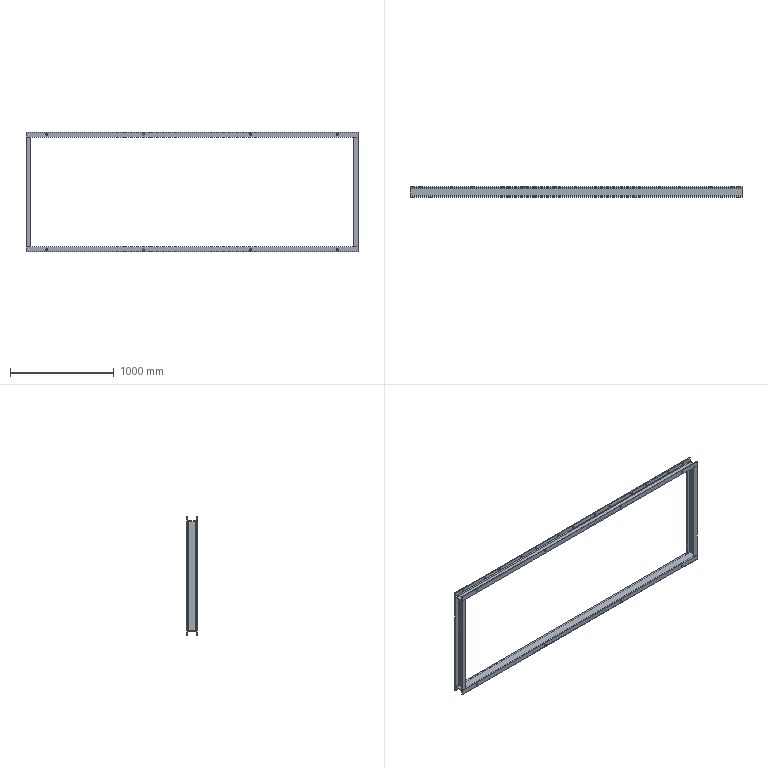Part | STEP file | SW-102-Base1_default<by machining> | 4 solids | 124 faces | box 3206 x 100 x 1155 mm | volume 10664759 mm3 | cylinder 84 | plane 40 | commonest cylinder face diameters 17.29 x52 18 x16 8.5 x8 17 x8